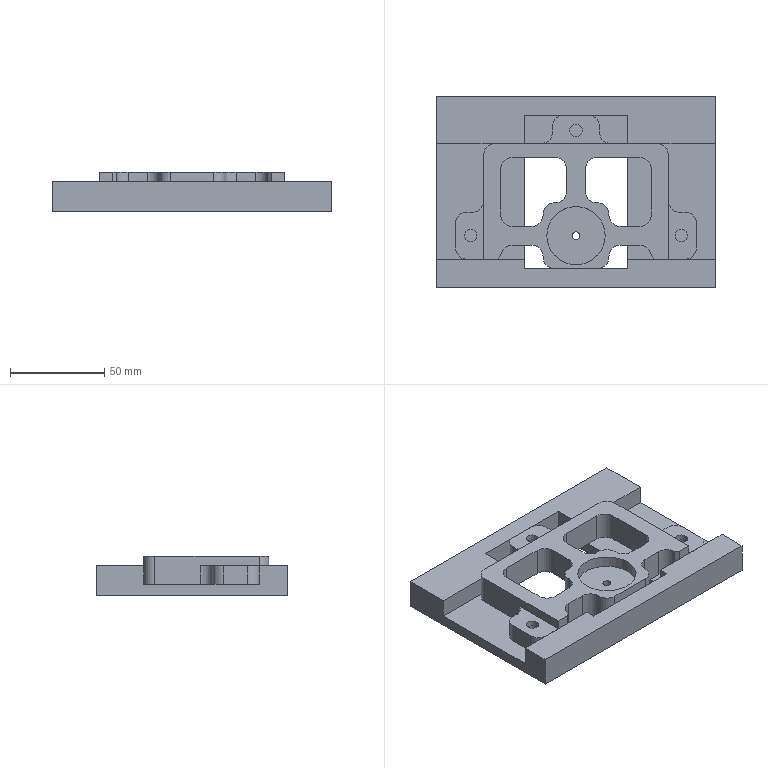NC program | NX | posted with a generic post | part box 148 x 101.5 x 21 mm
Lines 24 to 995 of 5700:
(ADAPTIVE_MILLING , TOOL : D10)
N46 T04 M6
N48 G54
N50 G17 G0 G90 X74.721 Y16.737 S9500 M3
N52 G43 Z30. H4
N54 Z-18.
N56 G94 G1 Z-21. F1000.
N58 X73.88 Y16.976 F3000.
N60 X73.034 Y17.191
N62 G3 X72.074 Y16.737 R1.021
N64 X71.38 Y14.348 R6.067
N66 X71.035 Y6.711 R67.293
N68 G1 X71.026 Y5.436
N70 X71.019 Y3.786
N72 X71.014 Y1.461
N74 X71.011 Y-2.439
N76 X71.01 Y-15.789
N78 Y-39.714
N80 G2 X68.668 Y-44.047 R5.611
N82 X63.36 Y-46.17 R11.767
N84 X55.06 Y-46.699 R55.713
N86 G1 X54.085 Y-46.71
N88 X52.886 Y-46.719
N90 X51.386 Y-46.726
N92 X49.436 Y-46.732
N94 X46.286 Y-46.736
N96 X39.236 Y-46.737
N98 X6.64 Y-46.738
N100 X6.523 Y-46.748
N102 X6.477 Y-46.75
N104 X-6.477
N106 X-6.523 Y-46.748
N108 X-7.648 Y-46.746
N110 X-8.548 Y-46.749
N112 X-9.298 Y-46.747
N114 X-10.348 Y-46.75
N116 X-11.248 Y-46.747
N118 X-11.998 Y-46.749
N120 X-13.198 Y-46.747
N122 X-13.873 Y-46.749
N124 X-15.148 Y-46.746
N126 X-15.898 Y-46.749
N128 X-16.873 Y-46.747
N130 X-17.473 Y-46.749
N132 X-18.523 Y-46.747
N134 X-18.898
N136 X-19.423 Y-46.749
N138 X-20.473 Y-46.747
N140 X-21.148 Y-46.749
N142 X-22.123 Y-46.747
N144 X-22.723 Y-46.749
N146 X-23.848 Y-46.747
N148 X-24.748 Y-46.749
N150 X-25.723 Y-46.747
N152 X-26.323 Y-46.749
N154 X-27.448 Y-46.748
N156 X-28.198 Y-46.75
N158 X-29.173 Y-46.747
N160 X-29.923 Y-46.749
N162 X-30.898 Y-46.748
N164 X-31.498 Y-46.749
N166 X-32.698 Y-46.747
N168 X-33.448 Y-46.749
N170 X-34.423 Y-46.747
N172 X-35.023 Y-46.749
N174 X-36.073 Y-46.747
N176 X-36.448 Y-46.746
N178 X-37.273 Y-46.749
N180 X-38.398 Y-46.746
N182 X-38.998 Y-46.748
N184 X-40.048 Y-46.747
N186 X-40.423
N188 X-40.948 Y-46.748
N190 X-41.923 Y-46.747
N192 X-42.598 Y-46.749
N194 X-43.723 Y-46.747
N196 X-44.473 Y-46.749
N198 X-45.373 Y-46.747
N200 X-46.198 Y-46.749
N202 X-47.023 Y-46.748
N204 X-47.998 Y-46.75
N206 X-48.823 Y-46.748
N208 X-49.948 Y-46.751
N210 X-50.548 Y-46.749
N212 X-51.748 Y-46.751
N214 X-52.423 Y-46.749
N216 X-53.398 Y-46.75
N218 X-54.073 Y-46.749
N220 G2 X-64.497 Y-46.718 R449.824
N222 X-68.686 Y-43.829 R6.104
N224 X-70.575 Y-38.032 R13.637
N226 X-70.969 Y-28.596 R84.882
N228 G1 X-70.976 Y-27.021
N230 X-70.982 Y-24.996
N232 X-70.985 Y-21.846
N234 X-70.987 Y-14.571
N236 Y39.729
N238 X-70.985 Y39.879
N240 G2 X-68.492 Y44.137 R5.755
N242 X-62.932 Y46.23 R12.384
N244 X-54.403 Y46.706 R62.969
N246 G1 X-53.353 Y46.716
N248 X-52.003 Y46.724
N250 X-50.203 Y46.73
N252 X-47.578 Y46.734
N254 X-42.703 Y46.737
N256 X-11.647
N258 X-11.523 Y46.748
N260 X-11.477 Y46.75
N262 X11.477
N264 X11.523 Y46.748
N266 X12.648
N268 X13.173 Y46.749
N270 X13.998 Y46.747
N272 X14.898 Y46.75
N274 X15.573 Y46.749
N276 X16.698 Y46.75
N278 X17.373 Y46.748
N280 X18.273 Y46.75
N282 X19.248 Y46.747
N284 X19.923 Y46.749
N286 X21.123 Y46.747
N288 X21.948 Y46.749
N290 X22.997 Y46.747
N292 X23.672 Y46.749
N294 X24.947 Y46.747
N296 X25.697 Y46.749
N298 X26.597 Y46.747
N300 X27.347 Y46.749
N302 X28.472 Y46.747
N304 X29.147 Y46.749
N306 X30.347 Y46.747
N308 X31.097 Y46.749
N310 X31.997 Y46.748
N312 X32.972 Y46.75
N314 X33.572 Y46.749
N316 X34.697 Y46.75
N318 X35.372 Y46.749
N320 X36.572 Y46.751
N322 X37.397 Y46.749
N324 X38.447 Y46.751
N326 X39.047 Y46.749
N328 X40.247 Y46.751
N330 X40.847 Y46.749
N332 X41.972 Y46.751
N334 X42.647 Y46.749
N336 X43.772 Y46.751
N338 X44.597 Y46.749
N340 X45.572 Y46.751
N342 X46.247 Y46.749
N344 X47.372 Y46.751
N346 X47.972 Y46.75
N348 X49.247 Y46.751
N350 X49.922 Y46.749
N352 X51.047 Y46.751
N354 X51.872 Y46.749
N356 X52.922 Y46.751
N358 X53.597 Y46.749
N360 X54.872 Y46.751
N362 X55.547 Y46.749
N364 X56.747 Y46.751
N366 X57.497 Y46.749
N368 X58.397 Y46.751
N370 X59.222 Y46.749
N372 X60.047 Y46.75
N374 G2 X64.62 Y46.7 R61.503
N376 X68.672 Y43.849 R6.141
N378 X70.553 Y38.205 R13.481
N380 X70.966 Y29.07 R77.812
N382 X70.94 Y19.396 R236.871
N384 G3 X70.233 Y12.006 R175.326
N386 X70.024 Y-4.266 R365.244
N388 G1 X70.022 Y-11.991
N390 Y-36.666
N392 X70.018 Y-36.891
N394 X70.012 Y-37.041
N396 X70.003 Y-37.19
N398 G2 X66.144 Y-43.2 R7.745
N400 X59.837 Y-45.231 R15.95
N402 X50.105 Y-45.697 R83.298
N404 G1 X48.68 Y-45.708
N406 X47.03 Y-45.715
N408 X44.78 Y-45.721
N410 X41.255 Y-45.724
N412 X33.08 Y-45.726
N414 X11.48
N416 G3 X10.559 Y-46.038 R2.719
N418 G2 X6.595 Y-46.742 R13.82
N420 G1 X8.629 Y-46.556
N422 X10.646 Y-46.007
N424 X11.096 Y-45.797
N426 G2 X13.884 Y-45.284 R8.319
N428 X25.507 Y-45.133 R226.361
N430 G1 X32.032 Y-45.132
N432 X33.382 Y-45.128
N434 X34.507
N436 X34.657
N438 X34.957
N440 X35.107
N442 X35.407
N444 X35.557
N446 X35.857
N448 X37.807 Y-45.126
N450 X38.182 Y-45.125
N452 X39.007
N454 X40.057 Y-45.124
N456 G3 X55.654 Y-44.945 R377.544
N458 X62.604 Y-43.883 R27.341
N460 X67.402 Y-40.484 R8.712
N462 X69.114 Y-35.1 R12.412
N464 X69.406 Y-26.935 R80.86
N466 G1 X69.411 Y-25.21
N468 X69.414 Y-22.285
N470 X69.416 Y-14.41
N472 X69.42 Y-13.135
N474 X69.419 Y-12.76
N476 Y-11.86
N478 Y-11.485
N480 X69.42 Y-9.535
N482 Y-9.16
N484 Y-7.885
N486 G2 X69.608 Y11.013 R516.518
N488 X70.228 Y18.562 R226.977
N490 G3 X70.163 Y35.43 R192.914
N492 X68.969 Y41.281 R17.97
N494 X64.758 Y45.005 R7.203
N496 X58.645 Y46.032 R19.894
N498 X42.296 Y46.146 R507.269
N500 G1 X39.146 Y46.145
N502 X38.921 Y46.146
N504 X31.421 Y46.144
N506 X29.921 Y46.147
N508 X29.246
N510 X28.646 Y46.146
N512 X28.196 Y46.147
N514 X27.596
N516 X26.921 Y46.145
N518 X26.471 Y46.147
N520 X26.096
N522 X25.121 Y46.146
N524 X24.521 Y46.148
N526 X24.221
N528 X23.171 Y46.146
N530 X22.796 Y46.147
N532 X20.621 Y46.149
N534 X20.171 Y46.15
N536 X19.721 Y46.149
N538 X18.821 Y46.151
N540 X18.371 Y46.149
N542 X18.221 Y46.15
N544 X17.921 Y46.149
N546 X17.246 Y46.151
N548 X16.346 Y46.148
N550 X15.521 Y46.15
N552 X15.296 Y46.149
N554 X15.221 Y46.152
N556 X15.147 Y46.16
N558 X15.095 Y46.169
N560 X13.577 Y46.565
N562 X13.488 Y46.58
N564 X11.523 Y46.748
N566 X13.488 Y46.58
N568 X13.577 Y46.565
N570 X15.095 Y46.169
N572 G3 X19.969 Y45.314 R15.754
N574 X36.017 Y45.155 R402.088
N576 G1 X36.617 Y45.152
N578 X37.592 Y45.151
N580 X38.117 Y45.152
N582 X38.792 Y45.149
N584 X39.767
N586 X40.517 Y45.147
N588 X41.492 Y45.149
N590 X42.092 Y45.147
N592 X43.292 Y45.148
N594 X43.667
N596 X44.117 Y45.147
N598 X45.317 Y45.148
N600 X45.992 Y45.146
N602 X47.117 Y45.147
N604 X47.792 Y45.145
N606 X48.842
N608 X49.517 Y45.143
N610 X50.567 Y45.142
N612 G2 X59.71 Y44.87 R103.638
N614 X64.142 Y43.593 R10.65
N616 X68.016 Y38.413 R9.552
N618 X68.906 Y34.649 R26.62
N620 G1 X69.257 Y33.896
N622 X69.288 Y33.809
N624 X69.806 Y31.879
N626 X69.822 Y31.788
N628 X69.998 Y29.773
N630 X70. Y29.727
N632 Y16.773
N634 X69.998 Y16.727
N636 X69.822 Y14.712
N638 X69.806 Y14.621
N640 G3 X68.575 Y6.671 R27.513
N642 X68.419 Y-16.577 R890.844
N644 G2 X68.291 Y-31.726 R449.873
N646 X67.386 Y-37.102 R17.357
N648 X62.3 Y-42.149 R9.457
N650 X55.169 Y-43.778 R21.851
N652 X42.802 Y-44.104 R162.371
N654 G1 X40.852 Y-44.109
N656 X40.402 Y-44.112
N658 X38.677 Y-44.118
N660 X37.027 Y-44.12
N662 X36.127
N664 X35.377 Y-44.124
N666 X34.402
N668 X33.877 Y-44.127
N670 X32.752
N672 X32.377
N674 X31.852 Y-44.129
N676 X30.802 Y-44.128
N678 X30.427
N680 X29.902 Y-44.13
N682 X28.702
N684 X28.102 Y-44.131
N686 X27.052 Y-44.13
N688 X26.302 Y-44.133
N690 X25.327 Y-44.132
N692 X24.652 Y-44.134
N694 X23.527
N696 G3 X14.082 Y-44.353 R127.202
N698 X13.363 Y-44.538 R1.944
N700 G2 X11.166 Y-45.764 R9.139
N702 G1 X12.458 Y-45.162
N704 X12.538 Y-45.116
N706 X13.363 Y-44.538
N708 G2 X15.495 Y-43.886 R4.877
N710 X23.133 Y-43.554 R65.613
N712 G1 X24.408 Y-43.548
N714 X28.083 Y-43.534
N716 X30.858 Y-43.526
N718 X31.233
N720 X32.058 Y-43.525
N722 X32.883 Y-43.526
N724 X34.308 Y-43.521
N726 X34.683 Y-43.522
N728 X35.433 Y-43.521
N730 X36.408 Y-43.519
N732 G3 X52.38 Y-43.326 R421.926
N734 X59.926 Y-42.204 R30.24
N736 X66.89 Y-35.004 R9.898
N738 X67.722 Y-28.021 R29.753
N740 X67.827 Y-8.147 R951.976
N742 G2 X68.04 Y7.45 R357.88
N744 X68.412 Y10.792 R17.568
N746 G1 X69.257 Y12.604
N748 X69.288 Y12.691
N750 X69.257 Y12.604
N752 X68.412 Y10.792
N754 X68.39 Y10.754
N756 G3 X67.409 Y7.894 R6.959
N758 X66.898 Y-0.408 R59.76
N760 G1 X66.884 Y-1.457
N762 X66.87 Y-2.732
N764 X66.858 Y-4.382
N766 X66.848 Y-6.257
N768 X66.84 Y-8.507
N770 X66.838 Y-9.032
N772 X66.835 Y-9.482
N774 X66.829 Y-11.057
N776 X66.827 Y-12.632
N778 X66.825 Y-13.007
N780 X66.823 Y-13.382
N782 X66.822 Y-14.582
N784 Y-15.182
N786 X66.817 Y-16.007
N788 Y-16.832
N790 X66.812 Y-17.732
N792 X66.811 Y-18.407
N794 X66.807 Y-19.382
N796 G2 X66.536 Y-30.251 R144.341
N798 X65.01 Y-36.01 R14.72
N800 X59.152 Y-40.791 R10.872
N802 X51.438 Y-42.228 R27.032
N804 X37.418 Y-42.502 R251.001
N806 G3 X19.119 Y-42.661 R660.553
N808 X15.108 Y-43.147 R18.581
N810 X14.175 Y-43.969 R4.752
N812 G1 X13.438 Y-44.485
N814 X14.175 Y-43.969
N816 X14.246 Y-43.91
N818 X14.847 Y-43.309
N820 G2 X16.538 Y-42.557 R3.385
N822 X22.654 Y-42.013 R32.743
N824 X39.903 Y-41.889 R936.917
N826 G3 X52.194 Y-41.521 R155.907
N828 X59.245 Y-39.877 R21.815
N830 X65.133 Y-32.884 R10.654
N832 X66.094 Y-25.466 R30.119
N834 X66.248 Y-6.342 R923.229
N836 G2 X66.563 Y5.426 R164.175
N838 X67.201 Y9.035 R16.114
N840 G1 X67.237 Y9.101
N842 X68.27 Y10.575
N844 X67.237 Y9.101
N846 G3 X66.08 Y6.559 R5.539
N848 X65.379 Y-0.369 R36.679
N850 X65.184 Y-19.718 R964.382
N852 G2 X64.745 Y-29.001 R76.656
N854 X62.532 Y-35.069 R13.291
N856 X56.123 Y-39.409 R12.326
N858 X47.991 Y-40.663 R33.113
N860 X31.044 Y-40.923 R426.642
N862 G3 X19.501 Y-41.223 R155.273
N864 X16.207 Y-41.893 R11.799
N866 X15.66 Y-42.496 R2.198
N868 G1 X14.917 Y-43.239
N870 X15.66 Y-42.496
N872 X15.719 Y-42.425
N874 X15.944 Y-42.104
N876 G2 X17.264 Y-41.297 R2.502
N878 X22.44 Y-40.518 R20.18
N880 X37.287 Y-40.287 R412.908
N882 G3 X49.653 Y-39.903 R166.664
N884 X57.009 Y-38.24 R23.545
N886 X63.488 Y-30.627 R11.408
N888 X64.478 Y-23.061 R32.101
N890 X64.694 Y-4.763 R986.923
N892 G2 X65.214 Y4.742 R76.843
N894 X66.087 Y7.909 R10.844
N896 G1 X66.131 Y7.969
N898 X66.141 Y7.985
N900 X67.149 Y8.993
N902 X66.141 Y7.985
N904 G3 X64.724 Y5.387 R5.32
N906 X63.869 Y-0.993 R29.7
N908 X63.591 Y-17.04 R524.74
N910 G2 X63.122 Y-26.623 R84.198
N912 X60.883 Y-33.003 R14.56
N914 X54.403 Y-37.625 R12.583
N916 X46.293 Y-39.002 R31.802
N918 X31.298 Y-39.322 R323.895
N920 G3 X21.108 Y-39.682 R130.712
N922 X17.107 Y-40.609 R12.93
N924 G1 X17.044 Y-40.649
N926 X16.984 Y-40.694
N928 X16.927 Y-40.743
N930 X16.873 Y-40.795
N932 X16.817 Y-40.857
N934 X16. Y-42.024
N936 X16.817 Y-40.857
N938 G2 X18.377 Y-39.857 R3.
N940 X23.836 Y-38.96 R20.578
N942 X36.432 Y-38.673 R306.677
N944 G3 X48.267 Y-38.185 R131.722
N946 X55.697 Y-36.227 R21.727
N948 X61.835 Y-28.558 R11.977
N950 X62.869 Y-20.695 R33.225
N952 X63.134 Y-5.398 R871.24
N954 G2 X63.766 Y3.422 R61.934
N956 X64.932 Y6.962 R10.209
N958 X65.852 Y7.696 R23.148
N960 G1 X65.746 Y7.59
N962 X65.675 Y7.531
N964 X65.056 Y7.097
N966 G3 X63.567 Y4.989 R4.18
N968 X62.411 Y-1.107 R22.06
N970 X62.037 Y-13.324 R216.323
N972 G2 X61.598 Y-23.661 R120.704
N974 X59.64 Y-30.381 R17.201
N976 X52.878 Y-35.804 R12.582
N978 X44.574 Y-37.348 R30.438
N980 X31.381 Y-37.73 R275.444
N982 G3 X21.872 Y-38.213 R95.621
N984 X17.716 Y-39.405 R11.686
N986 X17.342 Y-39.786 R3.22
N988 G1 X16.912 Y-40.708
N990 X16.866 Y-40.788
N992 X16.912 Y-40.708
N994 X17.342 Y-39.786
N996 G2 X18.565 Y-38.73 R2.391
N998 X23.423 Y-37.545 R14.869
N1000 X33.086 Y-37.111 R120.062
N1002 G3 X45.523 Y-36.624 R172.017
N1004 X53.091 Y-34.877 R24.932
N1006 X60.195 Y-26.561 R12.454
N1008 X61.25 Y-18.926 R33.385
N1010 X61.589 Y-5.806 R818.75
N1012 G2 X62.375 Y2.622 R50.251
N1014 X63.742 Y6.164 R9.422
N1016 G1 X63.796 Y6.217
N1018 X63.853 Y6.266
N1020 X63.912 Y6.311
N1022 X63.926 Y6.323
N1024 X63.958 Y6.338
N1026 X64.038 Y6.384
N1028 X64.837 Y6.944
N1030 X64.038 Y6.384
N1032 X63.958 Y6.338
N1034 X63.926 Y6.323
N1036 G3 X62.566 Y4.874 R3.063
N1038 X61.108 Y-0.219 R15.136
N1040 X60.51 Y-10.17 R94.005
N1042 G2 X60.005 Y-21.406 R149.833
N1044 X58.048 Y-28.363 R18.416
N1046 X50.941 Y-34.158 R12.933
N1048 X42.639 Y-35.72 R31.009
N1050 X30.648 Y-36.167 R308.143
N1052 G3 X22.204 Y-36.804 R63.843
N1054 X18.191 Y-38.189 R10.713
N1056 X17.757 Y-38.896 R1.332
N1058 G1 X17.376 Y-39.712
N1060 X17.757 Y-38.896
N1062 X17.788 Y-38.809
N1064 X17.814 Y-38.712
N1066 G2 X18.703 Y-37.649 R1.775
N1068 X23.084 Y-36.19 R11.561
N1070 X31.755 Y-35.551 R72.12
N1072 G3 X43.962 Y-34.953 R169.316
N1074 X51.636 Y-33.021 R23.989
N1076 X58.478 Y-24.906 R12.75
N1078 X59.64 Y-17.212 R32.672
N1080 X60.062 Y-5.895 R809.246
N1082 G2 X61.036 Y2.132 R40.981
N1084 X62.702 Y5.702 R8.678
N1086 X63.785 Y6.258 R7.036
N1088 G1 X62.902 Y5.846
N1090 G3 X61.191 Y4.124 R3.627
N1092 X59.593 Y-1.238 R15.863
N1094 X58.887 Y-11.483 R97.792
N1096 G2 X58.221 Y-20.754 R87.561
N1098 X55.642 Y-27.724 R16.114
N1100 X48.442 Y-32.734 R13.918
N1102 X39.958 Y-34.163 R35.418
N1104 X28.347 Y-34.714 R917.279
N1106 G3 X21.162 Y-35.749 R32.336
N1108 X18.319 Y-37.208 R7.122
N1110 G1 X18.273 Y-37.268
N1112 X18.231 Y-37.33
N1114 X18.194 Y-37.395
N1116 X18.161 Y-37.463
N1118 X18.132 Y-37.532
N1120 X18.127 Y-37.547
N1122 X17.835 Y-38.634
N1124 X18.127 Y-37.547
N1126 G2 X19.162 Y-36.313 R2.212
N1128 X23.873 Y-34.67 R12.29
N1130 X32.761 Y-33.919 R74.17
N1132 G3 X43.454 Y-33.152 R110.552
N1134 X50.914 Y-30.783 R20.716
N1136 X56.932 Y-22.776 R13.221
N1138 X58.077 Y-15.077 R35.619
N1140 G2 X58.694 Y-4.146 R424.21
N1142 X60.005 Y2.608 R26.478
N1144 X61.619 Y5.279 R6.772
N1146 G1 X61.682 Y5.319
N1148 X61.748 Y5.356
N1150 X61.816 Y5.388
N1152 X61.886 Y5.415
N1154 X62.059 Y5.462
N1156 X62.146 Y5.493
N1158 X62.69 Y5.747
N1160 X62.146 Y5.493
N1162 X62.059 Y5.462
N1164 X61.886 Y5.415
N1166 G3 X60.252 Y4.175 R2.815
N1168 X58.341 Y-0.674 R12.681
N1170 X57.378 Y-9.84 R63.367
N1172 G2 X56.594 Y-19.027 R92.525
N1174 X53.919 Y-26.041 R16.382
N1176 X48.958 Y-30.162 R13.711
N1178 X43.863 Y-31.851 R16.223
N1180 X34.768 Y-32.786 R69.209
N1182 G3 X24.83 Y-33.592 R109.512
N1184 X19.503 Y-35.289 R14.899
N1186 X18.414 Y-36.289 R2.651
N1188 G1 X18.388 Y-36.36
N1190 X18.366 Y-36.431
N1192 X18.349 Y-36.504
N1194 X18.344 Y-36.538
N1196 X18.322 Y-36.788
N1198 X18.306 Y-36.879
N1200 X18.15 Y-37.458
N1202 X18.306 Y-36.879
N1204 X18.322 Y-36.788
N1206 X18.344 Y-36.538
N1208 G2 X19.106 Y-35.299 R1.774
N1210 X23.24 Y-33.432 R10.17
N1212 X31.49 Y-32.398 R49.581
N1214 G3 X40.116 Y-31.75 R216.967
N1216 X45.129 Y-31.556 R33.992
N1218 G1 X47.012 Y-31.051
N1220 X45.038 Y-31.572
N1222 X42.977 Y-31.75
N1224 X29.016
N1226 X28.641 Y-31.769
N1228 G3 X21.311 Y-33.195 R23.59
N1230 X18.598 Y-35.012 R6.686
N1232 G1 X18.56 Y-35.077
N1234 X18.527 Y-35.144
N1236 X18.498 Y-35.214
N1238 X18.474 Y-35.285
N1240 X18.455 Y-35.357
N1242 X18.44 Y-35.431
N1244 X18.355 Y-36.402
N1246 X18.44 Y-35.431
N1248 G2 X19.215 Y-34.108 R1.994
N1250 X23.348 Y-32.071 R9.999
N1252 G1 X23.566 Y-32.013
N1254 X23.711 Y-31.975
N1256 X24.002 Y-31.904
N1258 X24.295 Y-31.837
N1260 X24.515 Y-31.789
N1262 X24.588 Y-31.774
N1264 X24.662 Y-31.76
N1266 X24.742 Y-31.75
N1268 X29.017
N1270 X24.742
N1272 G3 X21.339 Y-32.144 R9.107
N1274 X18.641 Y-33.959 R5.667
N1276 X18.498 Y-34.773 R1.663
N1278 G1 X18.452 Y-35.296
N1280 X18.498 Y-34.773
N1282 X18.5 Y-34.727
N1284 Y-34.427
N1286 G2 X19.2 Y-33.072 R1.824
N1288 X21.559 Y-31.75 R5.132
N1290 G1 X23.284
N1292 X21.559
N1294 G3 X18.594 Y-33.175 R3.233
N1296 X18.5 Y-34.293 R3.014
N1298 G1 Y-33.543
N1300 G2 X19.307 Y-32.179 R1.685
N1302 X20.221 Y-31.75 R1.898
N1304 G1 X21.046
N1306 X20.221
N1308 G3 X18.52 Y-32.806 R1.549
N1310 G1 X18.507 Y-32.88
N1312 X18.5 Y-32.955
N1314 Y-33.405
N1316 Y-32.955
N1318 G2 X19.939 Y-31.75 R1.228
N1320 G1 X19.639
N1322 X19.409 Y-31.78
N1324 G3 X18.573 Y-32.505 R1.084
N1326 G2 X20.33 Y-32.336 R1.002
N1328 G1 X20.484 Y-32.569
N1330 X21.589 Y-34.236 Z-20.9
N1332 G3 X22.47 Y-34.755 R1.027
N1334 G1 X43.487
N1336 G3 X46.444 Y-34.593 R28.594
N1338 G1 X47.918 Y-34.431
N1340 G3 X48.807 Y-33.375 R1.005
N1342 G1 X48.786 Y-33.03
N1344 X48.663 Y-31.033 Z-21.
N1346 G2 X49.083 Y-30.084 R1.021
N1348 G3 X52.219 Y-27.425 R13.654
N1350 X55.771 Y-19.337 R18.686
N1352 X56.736 Y-10.245 R68.777
N1354 G2 X57.705 Y-1.153 R71.694
N1356 X59.65 Y4.005 R13.947
N1358 X60.823 Y5.13 R2.909
N1360 G1 X61.619 Y5.344
N1362 X60.823 Y5.13
N1364 G3 X58.933 Y3.74 R3.278
N1366 X56.869 Y-1.288 R13.194
N1368 X55.763 Y-10.363 R65.894
N1370 G2 X55. Y-17.446 R90.236
N1372 X54.806 Y-21.879 R28.965
N1374 X53.412 Y-25.708 R13.931
N1376 G1 X54.288 Y-23.809
N1378 X54.822 Y-21.788
N1380 X55. Y-19.727
N1382 Y-17.446
N1384 G2 X56.145 Y-2.137 R80.785
N1386 X58.23 Y3.448 R15.374
N1388 X59.651 Y4.858 R3.92
N1390 G1 X59.722 Y4.882
N1392 X59.794 Y4.901
N1394 X59.868 Y4.913
N1396 X60.038 Y4.928
N1398 X60.129 Y4.944
N1400 X60.563 Y5.061
N1402 X60.129 Y4.944
N1404 X60.038 Y4.928
N1406 X59.868 Y4.913
N1408 G3 X58.124 Y3.992 R2.577
N1410 X55.755 Y-0.471 R10.88
N1412 X55. Y-3.758 R33.528
N1414 G1 Y-14.108
N1416 Y-3.758
N1418 G2 X57.526 Y3.895 R11.021
N1420 X58.846 Y4.824 R2.674
N1422 G1 X59.593 Y4.889
N1424 X58.846 Y4.824
N1426 G3 X56.843 Y3.765 R2.978
N1428 X55. Y0.623 R7.228
N1430 G1 Y-2.677
N1432 Y0.623
N1434 G2 X56.4 Y3.777 R4.903
N1436 X57.793 Y4.744 R2.707
N1438 G1 X57.868 Y4.75
N1440 X57.977
N1442 X58.023 Y4.752
N1444 X58.621 Y4.804
N1446 X58.023 Y4.752
N1448 X57.977 Y4.75
N1450 X57.868
N1452 G3 X55.896 Y3.818 R2.605
N1454 X55. Y2.379 R2.715
N1456 G1 Y0.729
N1458 Y2.379
N1460 G2 X56.055 Y4.288 R2.596
N1462 X57.577 Y4.75 R1.824
N1464 G1 X56.977
N1466 G3 X55.016 Y3.417 R1.947
N1468 G1 X55.005 Y3.343
N1470 X55. Y3.288
N1472 Y2.463
N1474 Y3.288
N1476 G2 X56.716 Y4.75 R1.491
N1478 G1 X56.266
N1480 G3 X55. Y3.386 R1.184
N1482 G2 X55.159 Y4.203 R1.551
N1484 X55.616 Y4.62 R1.093
N1486 X56.891 Y4.15 R1.005
N1488 G1 X57.228 Y3.209 Z-20.95
N1490 X57.549 Y2.262 Z-20.9
N1492 G3 X58.152 Y1.493 R1.125
N1494 X58.798 Y1.438 R1.041
N1496 G1 X62.431 Y2.358
N1498 G3 X66.255 Y4. R15.795
N1500 X68.303 Y5.672 R10.909
N1502 G1 X69.931 Y7.398
N1504 G3 X71.622 Y10.142 R11.023
N1506 X72.676 Y13.437 R17.235
N1508 X72.885 Y15.548 R12.327
N1510 G1 X72.997 Y29.024
N1512 G3 X72.803 Y32.399 R32.008
N1514 X72.044 Y33.284 R1.018
N1516 G1 X70.145 Y33.909 Z-21.
N1518 X69.349 Y34.186
N1520 G2 X68.906 Y34.649 R1.041
N1522 X67.394 Y38.243 R189.145
N1524 G3 X61.076 Y43.568 R9.476
N1526 X54.325 Y44.44 R27.732
N1528 X32.501 Y44.555 R992.858
N1530 G2 X19.98 Y44.753 R243.618
N1532 X17.607 Y45.067 R10.213
N1534 G3 X15.618 Y46.011 R26.575
N1536 G1 X17.325 Y45.237
N1538 X17.404 Y45.193
N1540 X17.537 Y45.102
N1542 G3 X20.332 Y44.094 R6.351
N1544 X28.261 Y43.613 R55.67
N1546 G1 X29.31 Y43.599
N1548 X30.51 Y43.588
N1550 X31.935 Y43.578
N1552 X33.81 Y43.57
N1554 X35.385 Y43.565
N1556 X35.985 Y43.561
N1558 X36.96 Y43.558
N1560 X37.485 Y43.557
N1562 X38.16 Y43.554
N1564 X39.285 Y43.552
N1566 X39.96 Y43.549
N1568 X41.01 Y43.548
N1570 X41.61 Y43.546
N1572 X42.66
N1574 X43.035 Y43.545
N1576 X43.56 Y43.543
N1578 X44.535 Y43.542
N1580 X45.51 Y43.537
N1582 X46.11
N1584 G2 X56.303 Y43.251 R126.003
N1586 X61.969 Y41.679 R14.01
N1588 X64.038 Y40.116 R16.025
N1590 X67.219 Y37.425 R13.85
N1592 G1 X68.366 Y35.788
N1594 X68.412 Y35.708
N1596 X68.602 Y35.3
N1598 X68.366 Y35.788
N1600 X67.16 Y37.496
N1602 X65.675 Y38.969
N1604 X63.982 Y40.148
N1606 G3 X54.413 Y42.686 R23.331
N1608 X41.443 Y42.943 R210.72
N1610 G2 X24.57 Y43.134 R486.85
N1612 X19.381 Y43.837 R21.825
N1614 G1 X19.315 Y43.871
N1616 X19.25 Y43.91
N1618 X19.189 Y43.952
N1620 X19.168 Y43.964
N1622 X19.088 Y44.041
N1624 X19.018 Y44.098
N1626 X17.901 Y44.856
N1628 X19.018 Y44.098
N1630 X19.088 Y44.041
N1632 X19.168 Y43.964
N1634 G3 X21.496 Y42.824 R4.808
N1636 X28.344 Y42.096 R33.483
N1638 X46.193 Y41.915 R877.894
N1640 G2 X52.472 Y41.75 R266.341
N1642 G1 X57.977
N1644 X58.023 Y41.748
N1646 X60.038 Y41.572
N1648 X60.129 Y41.556
N1650 X62.059 Y41.038
N1652 X62.146 Y41.007
N1654 X60.038 Y41.572
N1656 X57.977 Y41.75
N1658 X42.018
N1660 X41.951 Y41.746
N1662 G2 X34.766 Y41.412 R48.278
N1664 X24.204 Y41.816 R98.896
N1666 X20.502 Y42.711 R12.919
N1668 G1 X20.439 Y42.753
N1670 X20.38 Y42.799
N1672 X19.353 Y43.787
N1674 X20.38 Y42.799
N1676 G3 X22.935 Y41.412 R5.172
N1678 X29.392 Y40.576 R29.545
N1680 X38.312 Y40.53 R86.812
N1682 X39.155 Y41.032 R4.244
N1684 G2 X40.781 Y41.598 R7.061
N1686 G1 X40.43 Y41.537
N1688 X39.155 Y41.032
N1690 X38.879 Y40.855
N1692 X38.614 Y40.659
N1694 G2 X36.837 Y40.13 R3.773
N1696 X24.502 Y40.534 R49.44
N1698 X21.273 Y41.68 R8.846
N1700 G1 X21.218 Y41.731
N1702 X21.167 Y41.786
N1704 G2 X21.157 Y43.076 R1.108
N1706 X22.219 Y43.53 Z-20.939 R1.127
N1708 G1 X23.004 Y43.481 Z-20.9
N1710 X37.037 Y42.613
N1712 X38.073 Y42.538 Z-20.952
N1714 G2 X38.817 Y41.978 Z-21. R1.117
N1716 X38.493 Y40.571 R1.106
N1718 X35.981 Y39.669 R5.202
N1720 X24.261 Y40.074 R38.097
N1722 X21.807 Y40.964 R7.784
N1724 X20.553 Y42.621 R95.112
N1726 G1 X21.678 Y41.092
N1728 G3 X23.516 Y39.748 R3.667
N1730 X29.681 Y38.589 R19.661
N1732 X36.326 Y38.926 R24.394
N1734 X36.866 Y39.174 R1.992
N1736 G2 X38.267 Y40.407 R13.508
N1738 G1 X37.903 Y40.143
N1740 X37.852 Y40.1
N1742 X36.866 Y39.174
N1744 G2 X34.96 Y38.358 R3.826
N1746 X24.417 Y38.939 R23.774
N1748 X22.24 Y40.076 R6.057
N1750 X21.756 Y40.973 R25.472
N1752 G1 X22.138 Y40.209
N1754 G3 X23.94 Y38.587 R3.558
N1756 X30.126 Y37.227 R16.123
N1758 X35.255 Y37.683 R15.112
N1760 X35.9 Y38.267 R2.209
N1762 G1 X36.775 Y39.089
N1764 X35.9 Y38.267
N1766 X35.862 Y38.227
N1768 X35.589 Y37.912
N1770 G2 X33.94 Y37.087 R3.016
N1772 X24.232 Y37.986 R16.481
N1774 X22.712 Y39.05 R3.768
N1776 G1 X22.675 Y39.115
N1778 X22.668 Y39.127
N1780 X22.662 Y39.146
N1782 X22.629 Y39.229
N1784 X22.259 Y39.967
N1786 X22.629 Y39.229
N1788 X22.662 Y39.146
N1790 X22.668 Y39.127
N1792 G3 X24.036 Y37.595 R2.909
N1794 X29.684 Y36.001 R12.367
N1796 X34.416 Y36.537 R11.137
N1798 X35.107 Y37.355 R1.855
N1800 G1 X35.5 Y37.809
N1802 X35.107 Y37.355
N1804 X35.045 Y37.266
N1806 X34.859 Y36.931
N1808 G2 X33.683 Y36.061 R1.956
N1810 X27.976 Y35.746 R11.566
N1812 X23.443 Y37.588 R9.427
N1814 X22.944 Y38.213 R1.86
N1816 G1 X22.705 Y39.003
N1818 X22.944 Y38.213
N1820 G3 X24.422 Y36.396 R3.162
N1822 X33.241 Y35.225 R11.241
N1824 X34.388 Y36. R1.782
N1826 G1 X34.789 Y36.806
N1828 X34.498 Y36.281
N1830 X34.455 Y36.181
N1832 X34.421 Y36.07
N1834 G2 X33.384 Y35.059 R1.668
N1836 X28.378 Y34.541 R9.041
N1838 X23.738 Y36.481 R8.813
N1840 X23.227 Y37.279 R1.441
N1842 G1 X23.009 Y37.997
N1844 X23.227 Y37.279
N1846 X23.245 Y37.191
N1848 X23.249 Y37.158
N1850 G3 X24.224 Y35.612 R2.418
N1852 X26.865 Y34.25 R6.5
N1854 X32.339 Y34.282 R155.304
N1856 X34.024 Y35.01 R2.642
N1858 X34.395 Y35.988 R3.921
N1860 G1 X34.173 Y35.272
N1862 G2 X32.904 Y34.25 R1.496
N1864 G1 X31.929
N1866 X32.904
N1868 G3 X34.104 Y35.061 R1.162
N1870 G2 X33.003 Y34.25 R1.155
N1872 G1 X26.865
N1874 G2 X23.436 Y36.091 R4.235
N1876 X23.275 Y36.955 R4.44
N1878 G1 X23.348 Y36.36
N1880 G3 X25.14 Y34.259 R2.53
N1882 G1 X25.215 Y34.25
N1884 X26.715
N1886 X25.215
N1888 G2 X23.449 Y35.547 R1.917
N1890 G1 X23.385 Y36.068
N1892 X23.449 Y35.547
N1894 G3 X24.626 Y34.25 R1.289
N1896 G1 X25.076
N1898 X24.626
N1900 X24.436 Y34.275
N1902 G2 X23.486 Y35.27 R1.128
N1904 G1 X23.672 Y36.253
N1906 G2 X23.907 Y36.731 R1.062
N1908 G1 X24.141 Y36.994
N1910 X25.469 Y38.489 Z-20.9
N1912 X25.948 Y39.049
N1914 G3 X25.922 Y40.15 R1.01
N1916 G1 X24.146 Y42.718
N1918 X22.353 Y45.275
N1920 G3 X21.31 Y46.423 R6.29
N1922 X18.363 Y48.149 R13.441
N1924 G1 X17.212 Y48.62
N1926 X16.042 Y49.04
N1928 G3 X12.394 Y49.648 R14.037
N1930 G1 X-7.785 Y50.271
N1932 G3 X-8.58 Y49.917 R1.016
N1934 G1 X-9.13 Y49.265
N1936 X-10.42 Y47.736 Z-21.
N1938 X-10.935 Y47.126
N1940 X-10.967 Y47.089
N1942 G2 X-11.647 Y46.737 R1.112
N1944 G3 X-15.209 Y46.33 R54.705
N1946 G2 X-23.53 Y46.149 R124.748
N1948 G1 X-26.38 Y46.145
N1950 X-34.855 Y46.144
N1952 X-35.455 Y46.143
N1954 X-42.13
N1956 X-42.505 Y46.142
N1958 X-43.78
N1960 G3 X-58.628 Y45.978 R386.253
N1962 X-64.758 Y45.018 R23.003
N1964 X-69.193 Y40.644 R7.08
N1966 X-70.263 Y34.541 R19.156
N1968 X-70.381 Y18.342 R484.012
N1970 G1 Y-25.083
N1972 X-70.361 Y-28.908
N1974 G3 X-69.951 Y-37.518 R74.525
N1976 X-68.591 Y-42.011 R12.177
N1978 X-64.12 Y-45.225 R7.886
N1980 X-57.971 Y-46.059 R23.512
N1982 X-37.421 Y-46.15 R957.408